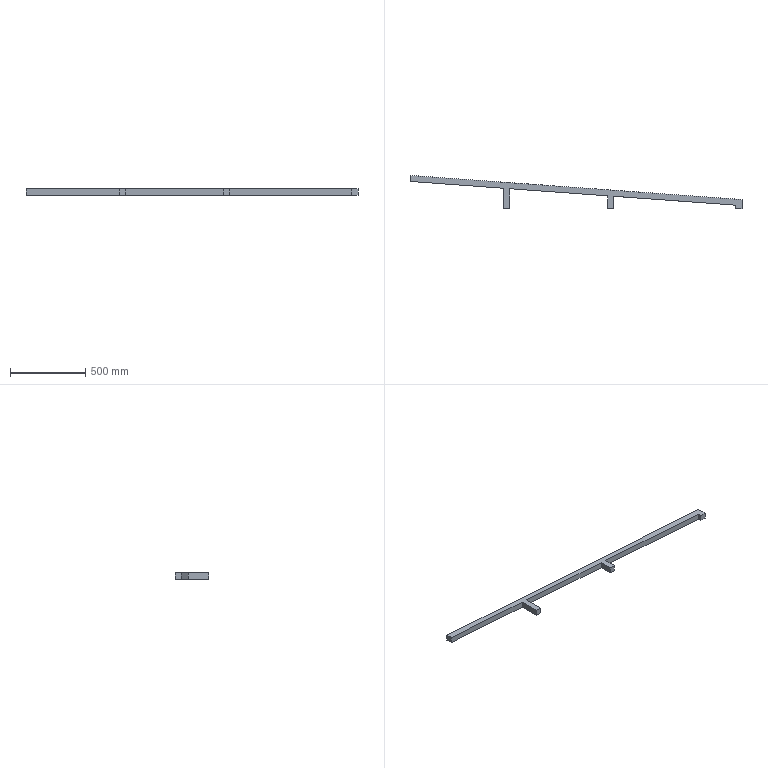Part | SolidWorks | features Extrusion 1 | 1 solid | 16 faces | box 2200 x 220 x 40 mm | volume 3909881 mm3 | plane 16
STEP:
#1=CARTESIAN_POINT('',(620.,134.803,0.));
#2=VERTEX_POINT('',#1);
#3=CARTESIAN_POINT('',(620.,0.,0.));
#4=VERTEX_POINT('',#3);
#5=CARTESIAN_POINT('',(620.,134.803,0.));
#6=DIRECTION('',(0.,-1.,0.));
#7=VECTOR('',#6,1000.);
#8=LINE('',#5,#7);
#9=EDGE_CURVE('',#2,#4,#8,.T.);
#10=ORIENTED_EDGE('',*,*,#9,.T.);
#11=CARTESIAN_POINT('',(620.,0.,40.));
#12=VERTEX_POINT('',#11);
#13=CARTESIAN_POINT('',(620.,0.,40.));
#14=DIRECTION('',(0.,0.,-1.));
#15=VECTOR('',#14,1000.);
#16=LINE('',#13,#15);
#17=EDGE_CURVE('',#12,#4,#16,.T.);
#18=ORIENTED_EDGE('',*,*,#17,.F.);
#19=CARTESIAN_POINT('',(620.,134.803,40.));
#20=VERTEX_POINT('',#19);
#21=CARTESIAN_POINT('',(620.,134.803,40.));
#22=DIRECTION('',(0.,-1.,0.));
#23=VECTOR('',#22,1000.);
#24=LINE('',#21,#23);
#25=EDGE_CURVE('',#20,#12,#24,.T.);
#26=ORIENTED_EDGE('',*,*,#25,.F.);
#27=CARTESIAN_POINT('',(620.,134.803,40.));
#28=DIRECTION('',(0.,0.,-1.));
#29=VECTOR('',#28,1000.);
#30=LINE('',#27,#29);
#31=EDGE_CURVE('',#20,#2,#30,.T.);
#32=ORIENTED_EDGE('',*,*,#31,.T.);
#33=EDGE_LOOP('',(#10,#18,#26,#32));
#34=FACE_OUTER_BOUND('',#33,.T.);
#35=CARTESIAN_POINT('',(620.,134.803,40.));
#36=DIRECTION('',(1.,0.,0.));
#37=DIRECTION('',(0.,1.,0.));
#38=AXIS2_PLACEMENT_3D('',#35,#36,#37);
#39=PLANE('',#38);
#40=ADVANCED_FACE('',(#34),#39,.F.);
#41=CARTESIAN_POINT('',(660.,0.,0.));
#42=VERTEX_POINT('',#41);
#43=CARTESIAN_POINT('',(620.,0.,0.));
#44=DIRECTION('',(1.,0.,0.));
#45=VECTOR('',#44,1000.);
#46=LINE('',#43,#45);
#47=EDGE_CURVE('',#4,#42,#46,.T.);
#48=ORIENTED_EDGE('',*,*,#47,.T.);
#49=CARTESIAN_POINT('',(660.,0.,40.));
#50=VERTEX_POINT('',#49);
#51=CARTESIAN_POINT('',(660.,0.,40.));
#52=DIRECTION('',(0.,0.,-1.));
#53=VECTOR('',#52,1000.);
#54=LINE('',#51,#53);
#55=EDGE_CURVE('',#50,#42,#54,.T.);
#56=ORIENTED_EDGE('',*,*,#55,.F.);
#57=CARTESIAN_POINT('',(620.,0.,40.));
#58=DIRECTION('',(1.,0.,0.));
#59=VECTOR('',#58,1000.);
#60=LINE('',#57,#59);
#61=EDGE_CURVE('',#12,#50,#60,.T.);
#62=ORIENTED_EDGE('',*,*,#61,.F.);
#63=ORIENTED_EDGE('',*,*,#17,.T.);
#64=EDGE_LOOP('',(#48,#56,#62,#63));
#65=FACE_OUTER_BOUND('',#64,.T.);
#66=CARTESIAN_POINT('',(620.,0.,40.));
#67=DIRECTION('',(0.,1.,0.));
#68=DIRECTION('',(-1.,0.,0.));
#69=AXIS2_PLACEMENT_3D('',#66,#67,#68);
#70=PLANE('',#69);
#71=ADVANCED_FACE('',(#65),#70,.F.);
#72=CARTESIAN_POINT('',(660.,131.894,0.));
#73=VERTEX_POINT('',#72);
#74=CARTESIAN_POINT('',(660.,131.894,0.));
#75=DIRECTION('',(0.,1.,0.));
#76=VECTOR('',#75,1000.);
#77=LINE('',#74,#76);
#78=EDGE_CURVE('',#42,#73,#77,.T.);
#79=ORIENTED_EDGE('',*,*,#78,.T.);
#80=CARTESIAN_POINT('',(660.,131.894,40.));
#81=VERTEX_POINT('',#80);
#82=CARTESIAN_POINT('',(660.,131.894,40.));
#83=DIRECTION('',(0.,0.,-1.));
#84=VECTOR('',#83,1000.);
#85=LINE('',#82,#84);
#86=EDGE_CURVE('',#81,#73,#85,.T.);
#87=ORIENTED_EDGE('',*,*,#86,.F.);
#88=CARTESIAN_POINT('',(660.,131.894,40.));
#89=DIRECTION('',(0.,1.,0.));
#90=VECTOR('',#89,1000.);
#91=LINE('',#88,#90);
#92=EDGE_CURVE('',#50,#81,#91,.T.);
#93=ORIENTED_EDGE('',*,*,#92,.F.);
#94=ORIENTED_EDGE('',*,*,#55,.T.);
#95=EDGE_LOOP('',(#79,#87,#93,#94));
#96=FACE_OUTER_BOUND('',#95,.T.);
#97=CARTESIAN_POINT('',(660.,131.894,40.));
#98=DIRECTION('',(-1.,0.,0.));
#99=DIRECTION('',(0.,0.,1.));
#100=AXIS2_PLACEMENT_3D('',#97,#98,#99);
#101=PLANE('',#100);
#102=ADVANCED_FACE('',(#96),#101,.F.);
#103=CARTESIAN_POINT('',(1310.,84.622,0.));
#104=VERTEX_POINT('',#103);
#105=CARTESIAN_POINT('',(660.,131.894,0.));
#106=DIRECTION('',(0.9974,-0.07254,0.));
#107=VECTOR('',#106,1000.);
#108=LINE('',#105,#107);
#109=EDGE_CURVE('',#73,#104,#108,.T.);
#110=ORIENTED_EDGE('',*,*,#109,.T.);
#111=CARTESIAN_POINT('',(1310.,84.622,40.));
#112=VERTEX_POINT('',#111);
#113=CARTESIAN_POINT('',(1310.,84.622,40.));
#114=DIRECTION('',(0.,0.,-1.));
#115=VECTOR('',#114,1000.);
#116=LINE('',#113,#115);
#117=EDGE_CURVE('',#112,#104,#116,.T.);
#118=ORIENTED_EDGE('',*,*,#117,.F.);
#119=CARTESIAN_POINT('',(660.,131.894,40.));
#120=DIRECTION('',(0.9974,-0.07254,0.));
#121=VECTOR('',#120,1000.);
#122=LINE('',#119,#121);
#123=EDGE_CURVE('',#81,#112,#122,.T.);
#124=ORIENTED_EDGE('',*,*,#123,.F.);
#125=ORIENTED_EDGE('',*,*,#86,.T.);
#126=EDGE_LOOP('',(#110,#118,#124,#125));
#127=FACE_OUTER_BOUND('',#126,.T.);
#128=CARTESIAN_POINT('',(660.,131.894,40.));
#129=DIRECTION('',(0.07254,0.9974,0.));
#130=DIRECTION('',(-0.9974,0.07254,0.));
#131=AXIS2_PLACEMENT_3D('',#128,#129,#130);
#132=PLANE('',#131);
#133=ADVANCED_FACE('',(#127),#132,.F.);
#134=CARTESIAN_POINT('',(1310.,0.,0.));
#135=VERTEX_POINT('',#134);
#136=CARTESIAN_POINT('',(1310.,84.622,0.));
#137=DIRECTION('',(0.,-1.,0.));
#138=VECTOR('',#137,1000.);
#139=LINE('',#136,#138);
#140=EDGE_CURVE('',#104,#135,#139,.T.);
#141=ORIENTED_EDGE('',*,*,#140,.T.);
#142=CARTESIAN_POINT('',(1310.,0.,40.));
#143=VERTEX_POINT('',#142);
#144=CARTESIAN_POINT('',(1310.,0.,40.));
#145=DIRECTION('',(0.,0.,-1.));
#146=VECTOR('',#145,1000.);
#147=LINE('',#144,#146);
#148=EDGE_CURVE('',#143,#135,#147,.T.);
#149=ORIENTED_EDGE('',*,*,#148,.F.);
#150=CARTESIAN_POINT('',(1310.,84.622,40.));
#151=DIRECTION('',(0.,-1.,0.));
#152=VECTOR('',#151,1000.);
#153=LINE('',#150,#152);
#154=EDGE_CURVE('',#112,#143,#153,.T.);
#155=ORIENTED_EDGE('',*,*,#154,.F.);
#156=ORIENTED_EDGE('',*,*,#117,.T.);
#157=EDGE_LOOP('',(#141,#149,#155,#156));
#158=FACE_OUTER_BOUND('',#157,.T.);
#159=CARTESIAN_POINT('',(1310.,84.622,40.));
#160=DIRECTION('',(1.,0.,0.));
#161=DIRECTION('',(0.,0.,-1.));
#162=AXIS2_PLACEMENT_3D('',#159,#160,#161);
#163=PLANE('',#162);
#164=ADVANCED_FACE('',(#158),#163,.F.);
#165=CARTESIAN_POINT('',(1350.,0.,0.));
#166=VERTEX_POINT('',#165);
#167=CARTESIAN_POINT('',(1310.,0.,0.));
#168=DIRECTION('',(1.,0.,0.));
#169=VECTOR('',#168,1000.);
#170=LINE('',#167,#169);
#171=EDGE_CURVE('',#135,#166,#170,.T.);
#172=ORIENTED_EDGE('',*,*,#171,.T.);
#173=CARTESIAN_POINT('',(1350.,0.,40.));
#174=VERTEX_POINT('',#173);
#175=CARTESIAN_POINT('',(1350.,0.,40.));
#176=DIRECTION('',(0.,0.,-1.));
#177=VECTOR('',#176,1000.);
#178=LINE('',#175,#177);
#179=EDGE_CURVE('',#174,#166,#178,.T.);
#180=ORIENTED_EDGE('',*,*,#179,.F.);
#181=CARTESIAN_POINT('',(1310.,0.,40.));
#182=DIRECTION('',(1.,0.,0.));
#183=VECTOR('',#182,1000.);
#184=LINE('',#181,#183);
#185=EDGE_CURVE('',#143,#174,#184,.T.);
#186=ORIENTED_EDGE('',*,*,#185,.F.);
#187=ORIENTED_EDGE('',*,*,#148,.T.);
#188=EDGE_LOOP('',(#172,#180,#186,#187));
#189=FACE_OUTER_BOUND('',#188,.T.);
#190=CARTESIAN_POINT('',(1310.,0.,40.));
#191=DIRECTION('',(0.,1.,0.));
#192=DIRECTION('',(0.,0.,1.));
#193=AXIS2_PLACEMENT_3D('',#190,#191,#192);
#194=PLANE('',#193);
#195=ADVANCED_FACE('',(#189),#194,.F.);
#196=CARTESIAN_POINT('',(1350.,81.713,0.));
#197=VERTEX_POINT('',#196);
#198=CARTESIAN_POINT('',(1350.,81.713,0.));
#199=DIRECTION('',(0.,1.,0.));
#200=VECTOR('',#199,1000.);
#201=LINE('',#198,#200);
#202=EDGE_CURVE('',#166,#197,#201,.T.);
#203=ORIENTED_EDGE('',*,*,#202,.T.);
#204=CARTESIAN_POINT('',(1350.,81.713,40.));
#205=VERTEX_POINT('',#204);
#206=CARTESIAN_POINT('',(1350.,81.713,40.));
#207=DIRECTION('',(0.,0.,-1.));
#208=VECTOR('',#207,1000.);
#209=LINE('',#206,#208);
#210=EDGE_CURVE('',#205,#197,#209,.T.);
#211=ORIENTED_EDGE('',*,*,#210,.F.);
#212=CARTESIAN_POINT('',(1350.,81.713,40.));
#213=DIRECTION('',(0.,1.,0.));
#214=VECTOR('',#213,1000.);
#215=LINE('',#212,#214);
#216=EDGE_CURVE('',#174,#205,#215,.T.);
#217=ORIENTED_EDGE('',*,*,#216,.F.);
#218=ORIENTED_EDGE('',*,*,#179,.T.);
#219=EDGE_LOOP('',(#203,#211,#217,#218));
#220=FACE_OUTER_BOUND('',#219,.T.);
#221=CARTESIAN_POINT('',(1350.,81.713,40.));
#222=DIRECTION('',(-1.,0.,0.));
#223=DIRECTION('',(0.,0.,1.));
#224=AXIS2_PLACEMENT_3D('',#221,#222,#223);
#225=PLANE('',#224);
#226=ADVANCED_FACE('',(#220),#225,.F.);
#227=CARTESIAN_POINT('',(2160.,22.803,0.));
#228=VERTEX_POINT('',#227);
#229=CARTESIAN_POINT('',(1350.,81.713,0.));
#230=DIRECTION('',(0.9974,-0.07254,0.));
#231=VECTOR('',#230,1000.);
#232=LINE('',#229,#231);
#233=EDGE_CURVE('',#197,#228,#232,.T.);
#234=ORIENTED_EDGE('',*,*,#233,.T.);
#235=CARTESIAN_POINT('',(2160.,22.803,40.));
#236=VERTEX_POINT('',#235);
#237=CARTESIAN_POINT('',(2160.,22.803,40.));
#238=DIRECTION('',(0.,0.,-1.));
#239=VECTOR('',#238,1000.);
#240=LINE('',#237,#239);
#241=EDGE_CURVE('',#236,#228,#240,.T.);
#242=ORIENTED_EDGE('',*,*,#241,.F.);
#243=CARTESIAN_POINT('',(1350.,81.713,40.));
#244=DIRECTION('',(0.9974,-0.07254,0.));
#245=VECTOR('',#244,1000.);
#246=LINE('',#243,#245);
#247=EDGE_CURVE('',#205,#236,#246,.T.);
#248=ORIENTED_EDGE('',*,*,#247,.F.);
#249=ORIENTED_EDGE('',*,*,#210,.T.);
#250=EDGE_LOOP('',(#234,#242,#248,#249));
#251=FACE_OUTER_BOUND('',#250,.T.);
#252=CARTESIAN_POINT('',(1350.,81.713,40.));
#253=DIRECTION('',(0.07254,0.9974,0.));
#254=DIRECTION('',(-0.9974,0.07254,0.));
#255=AXIS2_PLACEMENT_3D('',#252,#253,#254);
#256=PLANE('',#255);
#257=ADVANCED_FACE('',(#251),#256,.F.);
#258=CARTESIAN_POINT('',(2160.,0.,0.));
#259=VERTEX_POINT('',#258);
#260=CARTESIAN_POINT('',(2160.,22.803,0.));
#261=DIRECTION('',(0.,-1.,0.));
#262=VECTOR('',#261,1000.);
#263=LINE('',#260,#262);
#264=EDGE_CURVE('',#228,#259,#263,.T.);
#265=ORIENTED_EDGE('',*,*,#264,.T.);
#266=CARTESIAN_POINT('',(2160.,0.,40.));
#267=VERTEX_POINT('',#266);
#268=CARTESIAN_POINT('',(2160.,0.,40.));
#269=DIRECTION('',(0.,0.,-1.));
#270=VECTOR('',#269,1000.);
#271=LINE('',#268,#270);
#272=EDGE_CURVE('',#267,#259,#271,.T.);
#273=ORIENTED_EDGE('',*,*,#272,.F.);
#274=CARTESIAN_POINT('',(2160.,22.803,40.));
#275=DIRECTION('',(0.,-1.,0.));
#276=VECTOR('',#275,1000.);
#277=LINE('',#274,#276);
#278=EDGE_CURVE('',#236,#267,#277,.T.);
#279=ORIENTED_EDGE('',*,*,#278,.F.);
#280=ORIENTED_EDGE('',*,*,#241,.T.);
#281=EDGE_LOOP('',(#265,#273,#279,#280));
#282=FACE_OUTER_BOUND('',#281,.T.);
#283=CARTESIAN_POINT('',(2160.,22.803,40.));
#284=DIRECTION('',(1.,0.,0.));
#285=DIRECTION('',(0.,0.,-1.));
#286=AXIS2_PLACEMENT_3D('',#283,#284,#285);
#287=PLANE('',#286);
#288=ADVANCED_FACE('',(#282),#287,.F.);
#289=CARTESIAN_POINT('',(2200.,0.,0.));
#290=VERTEX_POINT('',#289);
#291=CARTESIAN_POINT('',(2160.,0.,0.));
#292=DIRECTION('',(1.,0.,0.));
#293=VECTOR('',#292,1000.);
#294=LINE('',#291,#293);
#295=EDGE_CURVE('',#259,#290,#294,.T.);
#296=ORIENTED_EDGE('',*,*,#295,.T.);
#297=CARTESIAN_POINT('',(2200.,0.,40.));
#298=VERTEX_POINT('',#297);
#299=CARTESIAN_POINT('',(2200.,0.,40.));
#300=DIRECTION('',(0.,0.,-1.));
#301=VECTOR('',#300,1000.);
#302=LINE('',#299,#301);
#303=EDGE_CURVE('',#298,#290,#302,.T.);
#304=ORIENTED_EDGE('',*,*,#303,.F.);
#305=CARTESIAN_POINT('',(2160.,0.,40.));
#306=DIRECTION('',(1.,0.,0.));
#307=VECTOR('',#306,1000.);
#308=LINE('',#305,#307);
#309=EDGE_CURVE('',#267,#298,#308,.T.);
#310=ORIENTED_EDGE('',*,*,#309,.F.);
#311=ORIENTED_EDGE('',*,*,#272,.T.);
#312=EDGE_LOOP('',(#296,#304,#310,#311));
#313=FACE_OUTER_BOUND('',#312,.T.);
#314=CARTESIAN_POINT('',(2160.,0.,40.));
#315=DIRECTION('',(0.,1.,0.));
#316=DIRECTION('',(0.,0.,1.));
#317=AXIS2_PLACEMENT_3D('',#314,#315,#316);
#318=PLANE('',#317);
#319=ADVANCED_FACE('',(#313),#318,.F.);
#320=CARTESIAN_POINT('',(2200.,60.,0.));
#321=VERTEX_POINT('',#320);
#322=CARTESIAN_POINT('',(2200.,0.,0.));
#323=DIRECTION('',(0.,1.,0.));
#324=VECTOR('',#323,1000.);
#325=LINE('',#322,#324);
#326=EDGE_CURVE('',#290,#321,#325,.T.);
#327=ORIENTED_EDGE('',*,*,#326,.T.);
#328=CARTESIAN_POINT('',(2200.,60.,40.));
#329=VERTEX_POINT('',#328);
#330=CARTESIAN_POINT('',(2200.,60.,40.));
#331=DIRECTION('',(0.,0.,-1.));
#332=VECTOR('',#331,1000.);
#333=LINE('',#330,#332);
#334=EDGE_CURVE('',#329,#321,#333,.T.);
#335=ORIENTED_EDGE('',*,*,#334,.F.);
#336=CARTESIAN_POINT('',(2200.,0.,40.));
#337=DIRECTION('',(0.,1.,0.));
#338=VECTOR('',#337,1000.);
#339=LINE('',#336,#338);
#340=EDGE_CURVE('',#298,#329,#339,.T.);
#341=ORIENTED_EDGE('',*,*,#340,.F.);
#342=ORIENTED_EDGE('',*,*,#303,.T.);
#343=EDGE_LOOP('',(#327,#335,#341,#342));
#344=FACE_OUTER_BOUND('',#343,.T.);
#345=CARTESIAN_POINT('',(2200.,0.,40.));
#346=DIRECTION('',(-1.,0.,0.));
#347=DIRECTION('',(0.,0.,1.));
#348=AXIS2_PLACEMENT_3D('',#345,#346,#347);
#349=PLANE('',#348);
#350=ADVANCED_FACE('',(#344),#349,.F.);
#351=CARTESIAN_POINT('',(0.,220.,0.));
#352=VERTEX_POINT('',#351);
#353=CARTESIAN_POINT('',(2200.,60.,0.));
#354=DIRECTION('',(-0.9974,0.07254,0.));
#355=VECTOR('',#354,1000.);
#356=LINE('',#353,#355);
#357=EDGE_CURVE('',#321,#352,#356,.T.);
#358=ORIENTED_EDGE('',*,*,#357,.T.);
#359=CARTESIAN_POINT('',(0.,220.,40.));
#360=VERTEX_POINT('',#359);
#361=CARTESIAN_POINT('',(0.,220.,40.));
#362=DIRECTION('',(0.,0.,-1.));
#363=VECTOR('',#362,1000.);
#364=LINE('',#361,#363);
#365=EDGE_CURVE('',#360,#352,#364,.T.);
#366=ORIENTED_EDGE('',*,*,#365,.F.);
#367=CARTESIAN_POINT('',(2200.,60.,40.));
#368=DIRECTION('',(-0.9974,0.07254,0.));
#369=VECTOR('',#368,1000.);
#370=LINE('',#367,#369);
#371=EDGE_CURVE('',#329,#360,#370,.T.);
#372=ORIENTED_EDGE('',*,*,#371,.F.);
#373=ORIENTED_EDGE('',*,*,#334,.T.);
#374=EDGE_LOOP('',(#358,#366,#372,#373));
#375=FACE_OUTER_BOUND('',#374,.T.);
#376=CARTESIAN_POINT('',(2200.,60.,40.));
#377=DIRECTION('',(-0.07254,-0.9974,0.));
#378=DIRECTION('',(0.9974,-0.07254,0.));
#379=AXIS2_PLACEMENT_3D('',#376,#377,#378);
#380=PLANE('',#379);
#381=ADVANCED_FACE('',(#375),#380,.F.);
#382=CARTESIAN_POINT('',(0.,179.894,0.));
#383=VERTEX_POINT('',#382);
#384=CARTESIAN_POINT('',(0.,220.,0.));
#385=DIRECTION('',(0.,-1.,0.));
#386=VECTOR('',#385,1000.);
#387=LINE('',#384,#386);
#388=EDGE_CURVE('',#352,#383,#387,.T.);
#389=ORIENTED_EDGE('',*,*,#388,.T.);
#390=CARTESIAN_POINT('',(0.,179.894,40.));
#391=VERTEX_POINT('',#390);
#392=CARTESIAN_POINT('',(0.,179.894,40.));
#393=DIRECTION('',(0.,0.,-1.));
#394=VECTOR('',#393,1000.);
#395=LINE('',#392,#394);
#396=EDGE_CURVE('',#391,#383,#395,.T.);
#397=ORIENTED_EDGE('',*,*,#396,.F.);
#398=CARTESIAN_POINT('',(0.,220.,40.));
#399=DIRECTION('',(0.,-1.,0.));
#400=VECTOR('',#399,1000.);
#401=LINE('',#398,#400);
#402=EDGE_CURVE('',#360,#391,#401,.T.);
#403=ORIENTED_EDGE('',*,*,#402,.F.);
#404=ORIENTED_EDGE('',*,*,#365,.T.);
#405=EDGE_LOOP('',(#389,#397,#403,#404));
#406=FACE_OUTER_BOUND('',#405,.T.);
#407=CARTESIAN_POINT('',(0.,220.,40.));
#408=DIRECTION('',(1.,0.,0.));
#409=DIRECTION('',(0.,1.,0.));
#410=AXIS2_PLACEMENT_3D('',#407,#408,#409);
#411=PLANE('',#410);
#412=ADVANCED_FACE('',(#406),#411,.F.);
#413=CARTESIAN_POINT('',(0.,179.894,0.));
#414=DIRECTION('',(0.9974,-0.07254,0.));
#415=VECTOR('',#414,1000.);
#416=LINE('',#413,#415);
#417=EDGE_CURVE('',#383,#2,#416,.T.);
#418=ORIENTED_EDGE('',*,*,#417,.T.);
#419=ORIENTED_EDGE('',*,*,#31,.F.);
#420=CARTESIAN_POINT('',(0.,179.894,40.));
#421=DIRECTION('',(0.9974,-0.07254,0.));
#422=VECTOR('',#421,1000.);
#423=LINE('',#420,#422);
#424=EDGE_CURVE('',#391,#20,#423,.T.);
#425=ORIENTED_EDGE('',*,*,#424,.F.);
#426=ORIENTED_EDGE('',*,*,#396,.T.);
#427=EDGE_LOOP('',(#418,#419,#425,#426));
#428=FACE_OUTER_BOUND('',#427,.T.);
#429=CARTESIAN_POINT('',(0.,179.894,40.));
#430=DIRECTION('',(0.07254,0.9974,0.));
#431=DIRECTION('',(-0.9974,0.07254,0.));
#432=AXIS2_PLACEMENT_3D('',#429,#430,#431);
#433=PLANE('',#432);
#434=ADVANCED_FACE('',(#428),#433,.F.);
#435=ORIENTED_EDGE('',*,*,#25,.T.);
#436=ORIENTED_EDGE('',*,*,#61,.T.);
#437=ORIENTED_EDGE('',*,*,#92,.T.);
#438=ORIENTED_EDGE('',*,*,#123,.T.);
#439=ORIENTED_EDGE('',*,*,#154,.T.);
#440=ORIENTED_EDGE('',*,*,#185,.T.);
#441=ORIENTED_EDGE('',*,*,#216,.T.);
#442=ORIENTED_EDGE('',*,*,#247,.T.);
#443=ORIENTED_EDGE('',*,*,#278,.T.);
#444=ORIENTED_EDGE('',*,*,#309,.T.);
#445=ORIENTED_EDGE('',*,*,#340,.T.);
#446=ORIENTED_EDGE('',*,*,#371,.T.);
#447=ORIENTED_EDGE('',*,*,#402,.T.);
#448=ORIENTED_EDGE('',*,*,#424,.T.);
#449=EDGE_LOOP('',(#435,#436,#437,#438,#439,#440,#441,#442,#443,#444,#445,#446,#447,#448));
#450=FACE_OUTER_BOUND('',#449,.T.);
#451=CARTESIAN_POINT('',(0.,0.,40.));
#452=DIRECTION('',(0.,0.,1.));
#453=DIRECTION('',(1.,0.,0.));
#454=AXIS2_PLACEMENT_3D('',#451,#452,#453);
#455=PLANE('',#454);
#456=ADVANCED_FACE('',(#450),#455,.T.);
#457=ORIENTED_EDGE('',*,*,#9,.F.);
#458=ORIENTED_EDGE('',*,*,#417,.F.);
#459=ORIENTED_EDGE('',*,*,#388,.F.);
#460=ORIENTED_EDGE('',*,*,#357,.F.);
#461=ORIENTED_EDGE('',*,*,#326,.F.);
#462=ORIENTED_EDGE('',*,*,#295,.F.);
#463=ORIENTED_EDGE('',*,*,#264,.F.);
#464=ORIENTED_EDGE('',*,*,#233,.F.);
#465=ORIENTED_EDGE('',*,*,#202,.F.);
#466=ORIENTED_EDGE('',*,*,#171,.F.);
#467=ORIENTED_EDGE('',*,*,#140,.F.);
#468=ORIENTED_EDGE('',*,*,#109,.F.);
#469=ORIENTED_EDGE('',*,*,#78,.F.);
#470=ORIENTED_EDGE('',*,*,#47,.F.);
#471=EDGE_LOOP('',(#457,#458,#459,#460,#461,#462,#463,#464,#465,#466,#467,#468,#469,#470));
#472=FACE_OUTER_BOUND('',#471,.T.);
#473=CARTESIAN_POINT('',(0.,0.,0.));
#474=DIRECTION('',(0.,0.,1.));
#475=DIRECTION('',(1.,0.,0.));
#476=AXIS2_PLACEMENT_3D('',#473,#474,#475);
#477=PLANE('',#476);
#478=ADVANCED_FACE('',(#472),#477,.F.);
#479=CLOSED_SHELL('',(#40,#71,#102,#133,#164,#195,#226,#257,#288,#319,#350,#381,#412,#434,#456,#478));
#480=MANIFOLD_SOLID_BREP('',#479);
#481=CARTESIAN_POINT('',(0.,0.,0.));
#482=DIRECTION('',(0.,0.,1.));
#483=DIRECTION('',(1.,0.,0.));
#484=AXIS2_PLACEMENT_3D('',#481,#482,#483);
#485=(LENGTH_UNIT()NAMED_UNIT(*)SI_UNIT(.MILLI.,.METRE.));
#486=UNCERTAINTY_MEASURE_WITH_UNIT(LENGTH_MEASURE(0.00001),#485,'','');
#487=(NAMED_UNIT(*)PLANE_ANGLE_UNIT()SI_UNIT($,.RADIAN.));
#488=(NAMED_UNIT(*)SI_UNIT($,.STERADIAN.)SOLID_ANGLE_UNIT());
#489=(GEOMETRIC_REPRESENTATION_CONTEXT(3)GLOBAL_UNCERTAINTY_ASSIGNED_CONTEXT((#486))GLOBAL_UNIT_ASSIGNED_CONTEXT((#485,#487,#488))REPRESENTATION_CONTEXT('',''));
#490=ADVANCED_BREP_SHAPE_REPRESENTATION('',(#480,#484),#489);